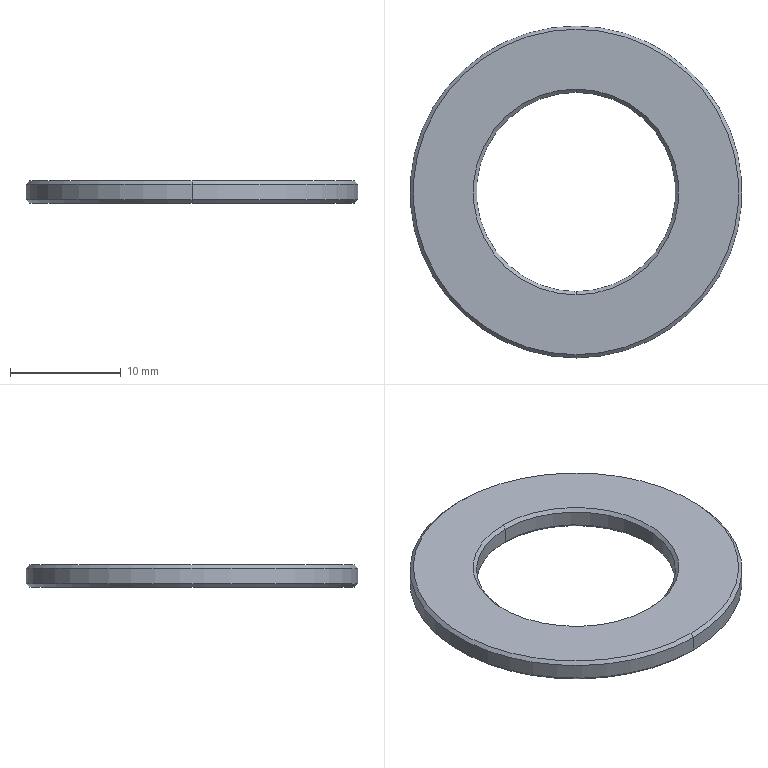Part | SolidWorks | features BaseBody 1 | 1 solid | 14 faces | box 30 x 30 x 2 mm | volume 891.207 mm3 | cone 8 | cylinder 4 | plane 2 | commonest cylinder face diameters 18 x2 30 x2
STEP:
#1=CARTESIAN_POINT('',(590.535,53.049,-63.23));
#2=VERTEX_POINT('',#1);
#3=CARTESIAN_POINT('',(590.535,23.649,-63.23));
#4=VERTEX_POINT('',#3);
#5=CARTESIAN_POINT('',(590.535,38.349,-63.23));
#6=DIRECTION('',(0.,0.,-1.));
#7=DIRECTION('',(0.,1.,0.));
#8=AXIS2_PLACEMENT_3D('',#5,#6,#7);
#9=CIRCLE('',#8,14.7);
#10=EDGE_CURVE('',#2,#4,#9,.T.);
#11=ORIENTED_EDGE('',*,*,#10,.T.);
#12=CARTESIAN_POINT('',(590.535,23.349,-63.53));
#13=VERTEX_POINT('',#12);
#14=CARTESIAN_POINT('',(590.535,23.349,-63.53));
#15=DIRECTION('',(0.,-0.7071,-0.7071));
#16=VECTOR('',#15,1000.);
#17=LINE('',#14,#16);
#18=EDGE_CURVE('',#4,#13,#17,.T.);
#19=ORIENTED_EDGE('',*,*,#18,.T.);
#20=CARTESIAN_POINT('',(590.535,53.349,-63.53));
#21=VERTEX_POINT('',#20);
#22=CARTESIAN_POINT('',(590.535,38.349,-63.53));
#23=DIRECTION('',(0.,0.,1.));
#24=DIRECTION('',(0.6374,0.7706,0.));
#25=AXIS2_PLACEMENT_3D('',#22,#23,#24);
#26=CIRCLE('',#25,15.);
#27=EDGE_CURVE('',#13,#21,#26,.T.);
#28=ORIENTED_EDGE('',*,*,#27,.T.);
#29=CARTESIAN_POINT('',(590.535,53.349,-63.53));
#30=DIRECTION('',(0.,0.7071,-0.7071));
#31=VECTOR('',#30,1000.);
#32=LINE('',#29,#31);
#33=EDGE_CURVE('',#2,#21,#32,.T.);
#34=ORIENTED_EDGE('',*,*,#33,.F.);
#35=EDGE_LOOP('',(#11,#19,#28,#34));
#36=FACE_OUTER_BOUND('',#35,.T.);
#37=CARTESIAN_POINT('',(590.535,38.349,-63.53));
#38=DIRECTION('',(0.,0.,-1.));
#39=DIRECTION('',(0.,1.,0.));
#40=AXIS2_PLACEMENT_3D('',#37,#38,#39);
#41=CONICAL_SURFACE('',#40,15.,0.7854);
#42=ADVANCED_FACE('',(#36),#41,.T.);
#43=CARTESIAN_POINT('',(590.535,47.349,-63.53));
#44=VERTEX_POINT('',#43);
#45=CARTESIAN_POINT('',(590.535,29.349,-63.53));
#46=VERTEX_POINT('',#45);
#47=CARTESIAN_POINT('',(590.535,38.349,-63.53));
#48=DIRECTION('',(0.,0.,1.));
#49=DIRECTION('',(0.6374,0.7706,0.));
#50=AXIS2_PLACEMENT_3D('',#47,#48,#49);
#51=CIRCLE('',#50,9.);
#52=EDGE_CURVE('',#44,#46,#51,.T.);
#53=ORIENTED_EDGE('',*,*,#52,.F.);
#54=CARTESIAN_POINT('',(590.535,47.649,-63.23));
#55=VERTEX_POINT('',#54);
#56=CARTESIAN_POINT('',(590.535,47.649,-63.23));
#57=DIRECTION('',(0.,0.7071,0.7071));
#58=VECTOR('',#57,1000.);
#59=LINE('',#56,#58);
#60=EDGE_CURVE('',#44,#55,#59,.T.);
#61=ORIENTED_EDGE('',*,*,#60,.T.);
#62=CARTESIAN_POINT('',(590.535,29.049,-63.23));
#63=VERTEX_POINT('',#62);
#64=CARTESIAN_POINT('',(590.535,38.349,-63.23));
#65=DIRECTION('',(0.,0.,1.));
#66=DIRECTION('',(0.,-1.,0.));
#67=AXIS2_PLACEMENT_3D('',#64,#65,#66);
#68=CIRCLE('',#67,9.3);
#69=EDGE_CURVE('',#55,#63,#68,.T.);
#70=ORIENTED_EDGE('',*,*,#69,.T.);
#71=CARTESIAN_POINT('',(590.535,29.049,-63.23));
#72=DIRECTION('',(0.,-0.7071,0.7071));
#73=VECTOR('',#72,1000.);
#74=LINE('',#71,#73);
#75=EDGE_CURVE('',#46,#63,#74,.T.);
#76=ORIENTED_EDGE('',*,*,#75,.F.);
#77=EDGE_LOOP('',(#53,#61,#70,#76));
#78=FACE_OUTER_BOUND('',#77,.T.);
#79=CARTESIAN_POINT('',(590.535,38.349,-63.23));
#80=DIRECTION('',(0.,0.,1.));
#81=DIRECTION('',(0.,-1.,0.));
#82=AXIS2_PLACEMENT_3D('',#79,#80,#81);
#83=CONICAL_SURFACE('',#82,9.3,0.7854);
#84=ADVANCED_FACE('',(#78),#83,.F.);
#85=ORIENTED_EDGE('',*,*,#27,.F.);
#86=CARTESIAN_POINT('',(590.535,23.349,-64.93));
#87=VERTEX_POINT('',#86);
#88=CARTESIAN_POINT('',(590.535,23.349,-63.23));
#89=DIRECTION('',(0.,0.,-1.));
#90=VECTOR('',#89,1000.);
#91=LINE('',#88,#90);
#92=EDGE_CURVE('',#13,#87,#91,.T.);
#93=ORIENTED_EDGE('',*,*,#92,.T.);
#94=CARTESIAN_POINT('',(590.535,53.349,-64.93));
#95=VERTEX_POINT('',#94);
#96=CARTESIAN_POINT('',(590.535,38.349,-64.93));
#97=DIRECTION('',(0.,0.,1.));
#98=DIRECTION('',(0.,1.,0.));
#99=AXIS2_PLACEMENT_3D('',#96,#97,#98);
#100=CIRCLE('',#99,15.);
#101=EDGE_CURVE('',#87,#95,#100,.T.);
#102=ORIENTED_EDGE('',*,*,#101,.T.);
#103=CARTESIAN_POINT('',(590.535,53.349,-63.23));
#104=DIRECTION('',(0.,0.,-1.));
#105=VECTOR('',#104,1000.);
#106=LINE('',#103,#105);
#107=EDGE_CURVE('',#21,#95,#106,.T.);
#108=ORIENTED_EDGE('',*,*,#107,.F.);
#109=EDGE_LOOP('',(#85,#93,#102,#108));
#110=FACE_OUTER_BOUND('',#109,.T.);
#111=CARTESIAN_POINT('',(590.535,38.349,-63.23));
#112=DIRECTION('',(0.,0.,-1.));
#113=DIRECTION('',(0.,1.,0.));
#114=AXIS2_PLACEMENT_3D('',#111,#112,#113);
#115=CYLINDRICAL_SURFACE('',#114,15.);
#116=ADVANCED_FACE('',(#110),#115,.T.);
#117=ORIENTED_EDGE('',*,*,#52,.T.);
#118=CARTESIAN_POINT('',(590.535,29.349,-64.93));
#119=VERTEX_POINT('',#118);
#120=CARTESIAN_POINT('',(590.535,29.349,-63.23));
#121=DIRECTION('',(0.,0.,-1.));
#122=VECTOR('',#121,1000.);
#123=LINE('',#120,#122);
#124=EDGE_CURVE('',#46,#119,#123,.T.);
#125=ORIENTED_EDGE('',*,*,#124,.T.);
#126=CARTESIAN_POINT('',(590.535,47.349,-64.93));
#127=VERTEX_POINT('',#126);
#128=CARTESIAN_POINT('',(590.535,38.349,-64.93));
#129=DIRECTION('',(0.,0.,1.));
#130=DIRECTION('',(0.,1.,0.));
#131=AXIS2_PLACEMENT_3D('',#128,#129,#130);
#132=CIRCLE('',#131,9.);
#133=EDGE_CURVE('',#127,#119,#132,.T.);
#134=ORIENTED_EDGE('',*,*,#133,.F.);
#135=CARTESIAN_POINT('',(590.535,47.349,-63.23));
#136=DIRECTION('',(0.,0.,-1.));
#137=VECTOR('',#136,1000.);
#138=LINE('',#135,#137);
#139=EDGE_CURVE('',#44,#127,#138,.T.);
#140=ORIENTED_EDGE('',*,*,#139,.F.);
#141=EDGE_LOOP('',(#117,#125,#134,#140));
#142=FACE_OUTER_BOUND('',#141,.T.);
#143=CARTESIAN_POINT('',(590.535,38.349,-63.23));
#144=DIRECTION('',(0.,0.,-1.));
#145=DIRECTION('',(0.,1.,0.));
#146=AXIS2_PLACEMENT_3D('',#143,#144,#145);
#147=CYLINDRICAL_SURFACE('',#146,9.);
#148=ADVANCED_FACE('',(#142),#147,.F.);
#149=CARTESIAN_POINT('',(590.535,23.649,-65.23));
#150=VERTEX_POINT('',#149);
#151=CARTESIAN_POINT('',(590.535,53.049,-65.23));
#152=VERTEX_POINT('',#151);
#153=CARTESIAN_POINT('',(590.535,38.349,-65.23));
#154=DIRECTION('',(0.,0.,1.));
#155=DIRECTION('',(0.,-1.,0.));
#156=AXIS2_PLACEMENT_3D('',#153,#154,#155);
#157=CIRCLE('',#156,14.7);
#158=EDGE_CURVE('',#150,#152,#157,.T.);
#159=ORIENTED_EDGE('',*,*,#158,.T.);
#160=CARTESIAN_POINT('',(590.535,53.349,-64.93));
#161=DIRECTION('',(0.,0.7071,0.7071));
#162=VECTOR('',#161,1000.);
#163=LINE('',#160,#162);
#164=EDGE_CURVE('',#152,#95,#163,.T.);
#165=ORIENTED_EDGE('',*,*,#164,.T.);
#166=ORIENTED_EDGE('',*,*,#101,.F.);
#167=CARTESIAN_POINT('',(590.535,23.349,-64.93));
#168=DIRECTION('',(0.,-0.7071,0.7071));
#169=VECTOR('',#168,1000.);
#170=LINE('',#167,#169);
#171=EDGE_CURVE('',#150,#87,#170,.T.);
#172=ORIENTED_EDGE('',*,*,#171,.F.);
#173=EDGE_LOOP('',(#159,#165,#166,#172));
#174=FACE_OUTER_BOUND('',#173,.T.);
#175=CARTESIAN_POINT('',(590.535,38.349,-64.93));
#176=DIRECTION('',(0.,0.,1.));
#177=DIRECTION('',(0.,-1.,0.));
#178=AXIS2_PLACEMENT_3D('',#175,#176,#177);
#179=CONICAL_SURFACE('',#178,15.,0.7854);
#180=ADVANCED_FACE('',(#174),#179,.T.);
#181=ORIENTED_EDGE('',*,*,#133,.T.);
#182=CARTESIAN_POINT('',(590.535,29.049,-65.23));
#183=VERTEX_POINT('',#182);
#184=CARTESIAN_POINT('',(590.535,29.049,-65.23));
#185=DIRECTION('',(0.,-0.7071,-0.7071));
#186=VECTOR('',#185,1000.);
#187=LINE('',#184,#186);
#188=EDGE_CURVE('',#119,#183,#187,.T.);
#189=ORIENTED_EDGE('',*,*,#188,.T.);
#190=CARTESIAN_POINT('',(590.535,47.649,-65.23));
#191=VERTEX_POINT('',#190);
#192=CARTESIAN_POINT('',(590.535,38.349,-65.23));
#193=DIRECTION('',(0.,0.,1.));
#194=DIRECTION('',(0.,1.,0.));
#195=AXIS2_PLACEMENT_3D('',#192,#193,#194);
#196=CIRCLE('',#195,9.3);
#197=EDGE_CURVE('',#191,#183,#196,.T.);
#198=ORIENTED_EDGE('',*,*,#197,.F.);
#199=CARTESIAN_POINT('',(590.535,47.649,-65.23));
#200=DIRECTION('',(0.,0.7071,-0.7071));
#201=VECTOR('',#200,1000.);
#202=LINE('',#199,#201);
#203=EDGE_CURVE('',#127,#191,#202,.T.);
#204=ORIENTED_EDGE('',*,*,#203,.F.);
#205=EDGE_LOOP('',(#181,#189,#198,#204));
#206=FACE_OUTER_BOUND('',#205,.T.);
#207=CARTESIAN_POINT('',(590.535,38.349,-65.23));
#208=DIRECTION('',(0.,0.,-1.));
#209=DIRECTION('',(0.,1.,0.));
#210=AXIS2_PLACEMENT_3D('',#207,#208,#209);
#211=CONICAL_SURFACE('',#210,9.3,0.7854);
#212=ADVANCED_FACE('',(#206),#211,.F.);
#213=ORIENTED_EDGE('',*,*,#10,.F.);
#214=CARTESIAN_POINT('',(590.535,38.349,-63.23));
#215=DIRECTION('',(0.,0.,-1.));
#216=DIRECTION('',(0.,1.,0.));
#217=AXIS2_PLACEMENT_3D('',#214,#215,#216);
#218=CIRCLE('',#217,14.7);
#219=EDGE_CURVE('',#4,#2,#218,.T.);
#220=ORIENTED_EDGE('',*,*,#219,.F.);
#221=EDGE_LOOP('',(#213,#220));
#222=FACE_OUTER_BOUND('',#221,.T.);
#223=CARTESIAN_POINT('',(590.535,38.349,-63.23));
#224=DIRECTION('',(0.,0.,1.));
#225=DIRECTION('',(0.,-1.,0.));
#226=AXIS2_PLACEMENT_3D('',#223,#224,#225);
#227=CIRCLE('',#226,9.3);
#228=EDGE_CURVE('',#63,#55,#227,.T.);
#229=ORIENTED_EDGE('',*,*,#228,.F.);
#230=ORIENTED_EDGE('',*,*,#69,.F.);
#231=EDGE_LOOP('',(#229,#230));
#232=FACE_BOUND('',#231,.T.);
#233=CARTESIAN_POINT('',(590.535,38.349,-63.23));
#234=DIRECTION('',(0.,0.,-1.));
#235=DIRECTION('',(0.,1.,0.));
#236=AXIS2_PLACEMENT_3D('',#233,#234,#235);
#237=PLANE('',#236);
#238=ADVANCED_FACE('',(#222,#232),#237,.F.);
#239=ORIENTED_EDGE('',*,*,#18,.F.);
#240=ORIENTED_EDGE('',*,*,#219,.T.);
#241=ORIENTED_EDGE('',*,*,#33,.T.);
#242=CARTESIAN_POINT('',(590.535,38.349,-63.53));
#243=DIRECTION('',(0.,0.,1.));
#244=DIRECTION('',(0.6374,0.7706,0.));
#245=AXIS2_PLACEMENT_3D('',#242,#243,#244);
#246=CIRCLE('',#245,15.);
#247=EDGE_CURVE('',#21,#13,#246,.T.);
#248=ORIENTED_EDGE('',*,*,#247,.T.);
#249=EDGE_LOOP('',(#239,#240,#241,#248));
#250=FACE_OUTER_BOUND('',#249,.T.);
#251=CARTESIAN_POINT('',(590.535,38.349,-63.53));
#252=DIRECTION('',(0.,0.,-1.));
#253=DIRECTION('',(0.,1.,0.));
#254=AXIS2_PLACEMENT_3D('',#251,#252,#253);
#255=CONICAL_SURFACE('',#254,15.,0.7854);
#256=ADVANCED_FACE('',(#250),#255,.T.);
#257=ORIENTED_EDGE('',*,*,#60,.F.);
#258=CARTESIAN_POINT('',(590.535,38.349,-63.53));
#259=DIRECTION('',(0.,0.,1.));
#260=DIRECTION('',(0.6374,0.7706,0.));
#261=AXIS2_PLACEMENT_3D('',#258,#259,#260);
#262=CIRCLE('',#261,9.);
#263=EDGE_CURVE('',#46,#44,#262,.T.);
#264=ORIENTED_EDGE('',*,*,#263,.F.);
#265=ORIENTED_EDGE('',*,*,#75,.T.);
#266=ORIENTED_EDGE('',*,*,#228,.T.);
#267=EDGE_LOOP('',(#257,#264,#265,#266));
#268=FACE_OUTER_BOUND('',#267,.T.);
#269=CARTESIAN_POINT('',(590.535,38.349,-63.23));
#270=DIRECTION('',(0.,0.,1.));
#271=DIRECTION('',(0.,-1.,0.));
#272=AXIS2_PLACEMENT_3D('',#269,#270,#271);
#273=CONICAL_SURFACE('',#272,9.3,0.7854);
#274=ADVANCED_FACE('',(#268),#273,.F.);
#275=ORIENTED_EDGE('',*,*,#92,.F.);
#276=ORIENTED_EDGE('',*,*,#247,.F.);
#277=ORIENTED_EDGE('',*,*,#107,.T.);
#278=CARTESIAN_POINT('',(590.535,38.349,-64.93));
#279=DIRECTION('',(0.,0.,1.));
#280=DIRECTION('',(0.,1.,0.));
#281=AXIS2_PLACEMENT_3D('',#278,#279,#280);
#282=CIRCLE('',#281,15.);
#283=EDGE_CURVE('',#95,#87,#282,.T.);
#284=ORIENTED_EDGE('',*,*,#283,.T.);
#285=EDGE_LOOP('',(#275,#276,#277,#284));
#286=FACE_OUTER_BOUND('',#285,.T.);
#287=CARTESIAN_POINT('',(590.535,38.349,-63.23));
#288=DIRECTION('',(0.,0.,-1.));
#289=DIRECTION('',(0.,1.,0.));
#290=AXIS2_PLACEMENT_3D('',#287,#288,#289);
#291=CYLINDRICAL_SURFACE('',#290,15.);
#292=ADVANCED_FACE('',(#286),#291,.T.);
#293=ORIENTED_EDGE('',*,*,#124,.F.);
#294=ORIENTED_EDGE('',*,*,#263,.T.);
#295=ORIENTED_EDGE('',*,*,#139,.T.);
#296=CARTESIAN_POINT('',(590.535,38.349,-64.93));
#297=DIRECTION('',(0.,0.,1.));
#298=DIRECTION('',(0.,1.,0.));
#299=AXIS2_PLACEMENT_3D('',#296,#297,#298);
#300=CIRCLE('',#299,9.);
#301=EDGE_CURVE('',#119,#127,#300,.T.);
#302=ORIENTED_EDGE('',*,*,#301,.F.);
#303=EDGE_LOOP('',(#293,#294,#295,#302));
#304=FACE_OUTER_BOUND('',#303,.T.);
#305=CARTESIAN_POINT('',(590.535,38.349,-63.23));
#306=DIRECTION('',(0.,0.,-1.));
#307=DIRECTION('',(0.,1.,0.));
#308=AXIS2_PLACEMENT_3D('',#305,#306,#307);
#309=CYLINDRICAL_SURFACE('',#308,9.);
#310=ADVANCED_FACE('',(#304),#309,.F.);
#311=ORIENTED_EDGE('',*,*,#164,.F.);
#312=CARTESIAN_POINT('',(590.535,38.349,-65.23));
#313=DIRECTION('',(0.,0.,1.));
#314=DIRECTION('',(0.,-1.,0.));
#315=AXIS2_PLACEMENT_3D('',#312,#313,#314);
#316=CIRCLE('',#315,14.7);
#317=EDGE_CURVE('',#152,#150,#316,.T.);
#318=ORIENTED_EDGE('',*,*,#317,.T.);
#319=ORIENTED_EDGE('',*,*,#171,.T.);
#320=ORIENTED_EDGE('',*,*,#283,.F.);
#321=EDGE_LOOP('',(#311,#318,#319,#320));
#322=FACE_OUTER_BOUND('',#321,.T.);
#323=CARTESIAN_POINT('',(590.535,38.349,-64.93));
#324=DIRECTION('',(0.,0.,1.));
#325=DIRECTION('',(0.,-1.,0.));
#326=AXIS2_PLACEMENT_3D('',#323,#324,#325);
#327=CONICAL_SURFACE('',#326,15.,0.7854);
#328=ADVANCED_FACE('',(#322),#327,.T.);
#329=ORIENTED_EDGE('',*,*,#188,.F.);
#330=ORIENTED_EDGE('',*,*,#301,.T.);
#331=ORIENTED_EDGE('',*,*,#203,.T.);
#332=CARTESIAN_POINT('',(590.535,38.349,-65.23));
#333=DIRECTION('',(0.,0.,1.));
#334=DIRECTION('',(0.,1.,0.));
#335=AXIS2_PLACEMENT_3D('',#332,#333,#334);
#336=CIRCLE('',#335,9.3);
#337=EDGE_CURVE('',#183,#191,#336,.T.);
#338=ORIENTED_EDGE('',*,*,#337,.F.);
#339=EDGE_LOOP('',(#329,#330,#331,#338));
#340=FACE_OUTER_BOUND('',#339,.T.);
#341=CARTESIAN_POINT('',(590.535,38.349,-65.23));
#342=DIRECTION('',(0.,0.,-1.));
#343=DIRECTION('',(0.,1.,0.));
#344=AXIS2_PLACEMENT_3D('',#341,#342,#343);
#345=CONICAL_SURFACE('',#344,9.3,0.7854);
#346=ADVANCED_FACE('',(#340),#345,.F.);
#347=ORIENTED_EDGE('',*,*,#197,.T.);
#348=ORIENTED_EDGE('',*,*,#337,.T.);
#349=EDGE_LOOP('',(#347,#348));
#350=FACE_BOUND('',#349,.T.);
#351=ORIENTED_EDGE('',*,*,#158,.F.);
#352=ORIENTED_EDGE('',*,*,#317,.F.);
#353=EDGE_LOOP('',(#351,#352));
#354=FACE_OUTER_BOUND('',#353,.T.);
#355=CARTESIAN_POINT('',(590.535,38.349,-65.23));
#356=DIRECTION('',(0.,0.,-1.));
#357=DIRECTION('',(0.,1.,0.));
#358=AXIS2_PLACEMENT_3D('',#355,#356,#357);
#359=PLANE('',#358);
#360=ADVANCED_FACE('',(#350,#354),#359,.T.);
#361=CLOSED_SHELL('',(#42,#84,#116,#148,#180,#212,#238,#256,#274,#292,#310,#328,#346,#360));
#362=MANIFOLD_SOLID_BREP('',#361);
#363=CARTESIAN_POINT('',(0.,0.,0.));
#364=DIRECTION('',(0.,0.,1.));
#365=DIRECTION('',(1.,0.,0.));
#366=AXIS2_PLACEMENT_3D('',#363,#364,#365);
#367=(LENGTH_UNIT()NAMED_UNIT(*)SI_UNIT(.MILLI.,.METRE.));
#368=UNCERTAINTY_MEASURE_WITH_UNIT(LENGTH_MEASURE(0.00001),#367,'','');
#369=(NAMED_UNIT(*)PLANE_ANGLE_UNIT()SI_UNIT($,.RADIAN.));
#370=(NAMED_UNIT(*)SI_UNIT($,.STERADIAN.)SOLID_ANGLE_UNIT());
#371=(GEOMETRIC_REPRESENTATION_CONTEXT(3)GLOBAL_UNCERTAINTY_ASSIGNED_CONTEXT((#368))GLOBAL_UNIT_ASSIGNED_CONTEXT((#367,#369,#370))REPRESENTATION_CONTEXT('',''));
#372=ADVANCED_BREP_SHAPE_REPRESENTATION('',(#362,#366),#371);